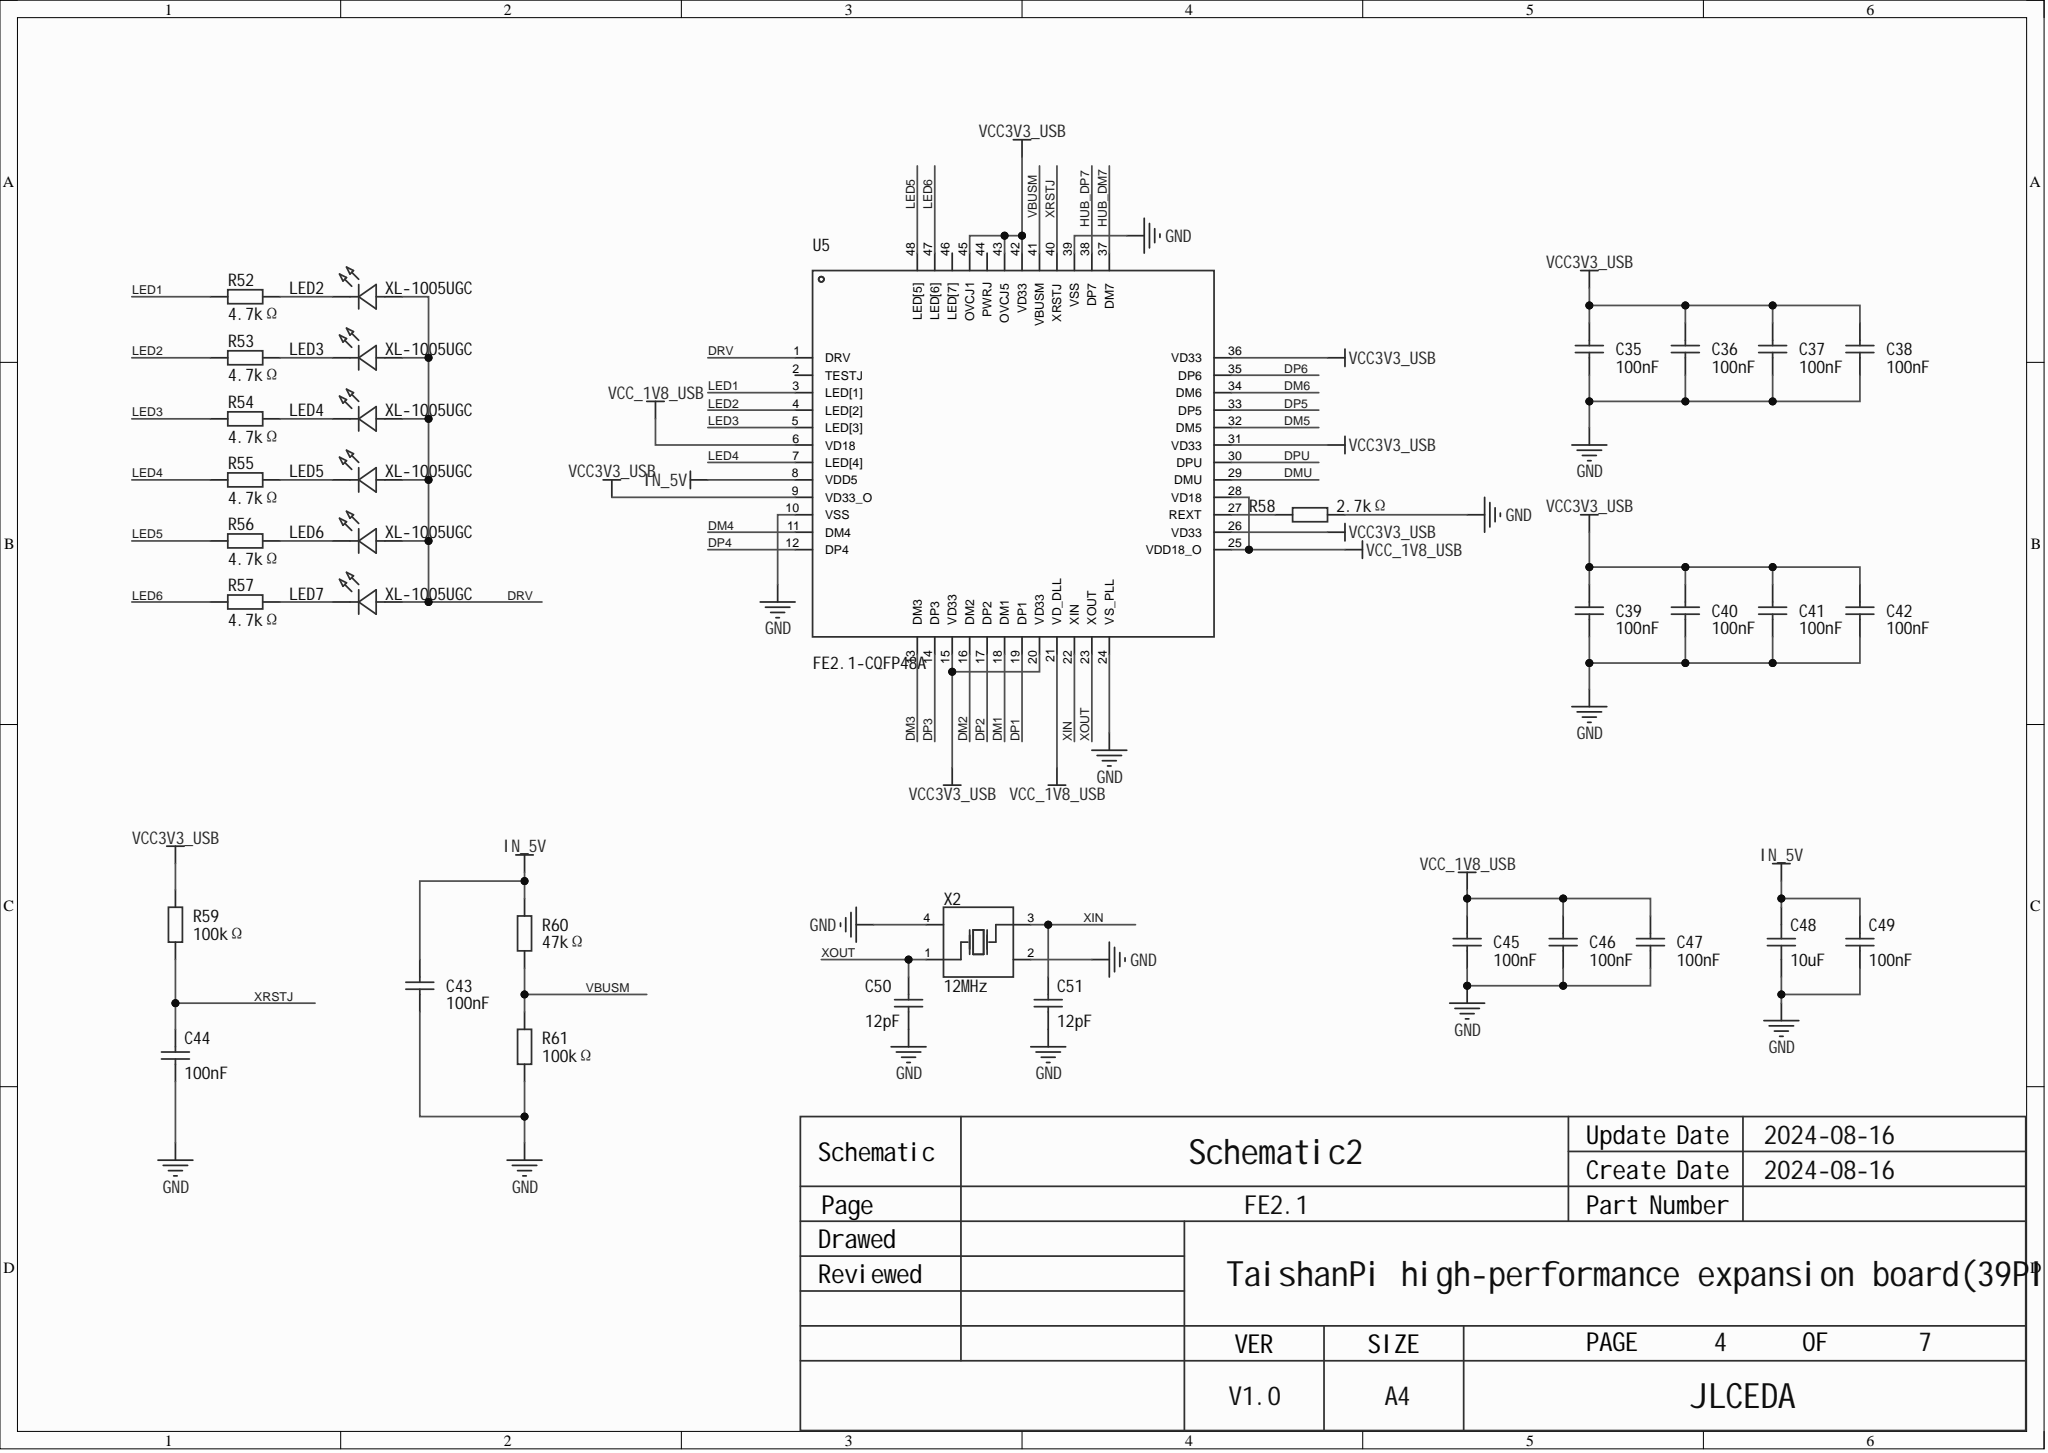Circuit board | Altium Designer | 209 parts | 149 nets | one sheet of the schematic
Parts on this sheet (reference | value | footprint):
C35 | 100nF | R0402
C36 | 100nF | R0402
C37 | 100nF | R0402
C38 | 100nF | R0402
C39 | 100nF | R0402
C40 | 100nF | R0402
C41 | 100nF | R0402
C42 | 100nF | R0402
C43 | 100nF | R0402
C44 | 100nF | R0402
C45 | 100nF | R0402
C46 | 100nF | R0402
C47 | 100nF | R0402
C48 | 10uF | r0603
C49 | 100nF | R0402
C50 | 12pF | R0402
C51 | 12pF | R0402
LED2 | XL-1005UGC | LED0402-RD_GREEN
LED3 | XL-1005UGC | LED0402-RD_GREEN
LED4 | XL-1005UGC | LED0402-RD_GREEN
LED5 | XL-1005UGC | LED0402-RD_GREEN
LED6 | XL-1005UGC | LED0402-RD_GREEN
LED7 | XL-1005UGC | LED0402-RD_GREEN
R52 | 4.7kΩ | R0402
R53 | 4.7kΩ | R0402
R54 | 4.7kΩ | R0402
R55 | 4.7kΩ | R0402
R56 | 4.7kΩ | R0402
R57 | 4.7kΩ | R0402
R58 | 2.7kΩ | R0402
R59 | 100kΩ | R0402
R60 | 47kΩ | R0402
R61 | 100kΩ | R0402
U5 | FE2.1-CQFP48A | LQFP-48_L7.0-W7.0-P0.50-LS9.0-BL
X2 | 12MHz | OSC-SMD_4P-L3.2-W2.5-BL
Nets of these parts (net: part-pin ...):
XRSTJ: C44-2 R59-1 U5-40
XOUT: C50-2 X2-1 U5-23
XIN: C51-1 X2-3 U5-22
VCC_1V8_USB: C45-2 C46-2 C47-2 U5-6 U5-21 U5-25 U5-28
VCC3V3_USB: C35-2 C36-2 C37-2 C38-2 C39-2 C40-2 C41-2 C42-2 R59-2 U5-9 U5-15 U5-20 U5-26 U5-31 U5-36 U5-42 U5-43 U5-45
VBUSM: R60-1 R61-2 U5-41
NetR58_1: R58-1 U5-27
NetLED7_1: LED7-1 R57-1
NetLED6_1: LED6-1 R56-1
NetLED5_1: LED5-1 R55-1
NetLED4_1: LED4-1 R54-1
NetLED3_1: LED3-1 R53-1
NetLED2_1: LED2-1 R52-1
LED6: R57-2 U5-47
LED5: R56-2
LED4: R55-2 U5-7
LED3: R54-2 U5-5
LED2: R53-2 U5-4
LED1: R52-2 U5-3
IN_5V: C43-2 C48-2 C49-2 R60-2 U5-8
HUB_DP7: U5-38
HUB_DM7: U5-37
GND: C35-1 C36-1 C37-1 C38-1 C39-1 C40-1 C41-1 C42-1 C43-1 C44-1 C45-1 C46-1 C47-1 C48-1 C49-1 C50-1 C51-2 R58-2 R61-1 X2-2 X2-4 U5-10 U5-24 U5-39
DRV: LED2-2 LED3-2 LED4-2 LED5-2 LED6-2 LED7-2 U5-1
DPU: U5-30
DP6: U5-35
DP5: U5-33
DP4: U5-12
DP3: U5-14
DP2: U5-17
DP1: U5-19
DMU: U5-29
DM6: U5-34
DM5: U5-32
DM4: U5-11
DM3: U5-13
DM2: U5-16
DM1: U5-18